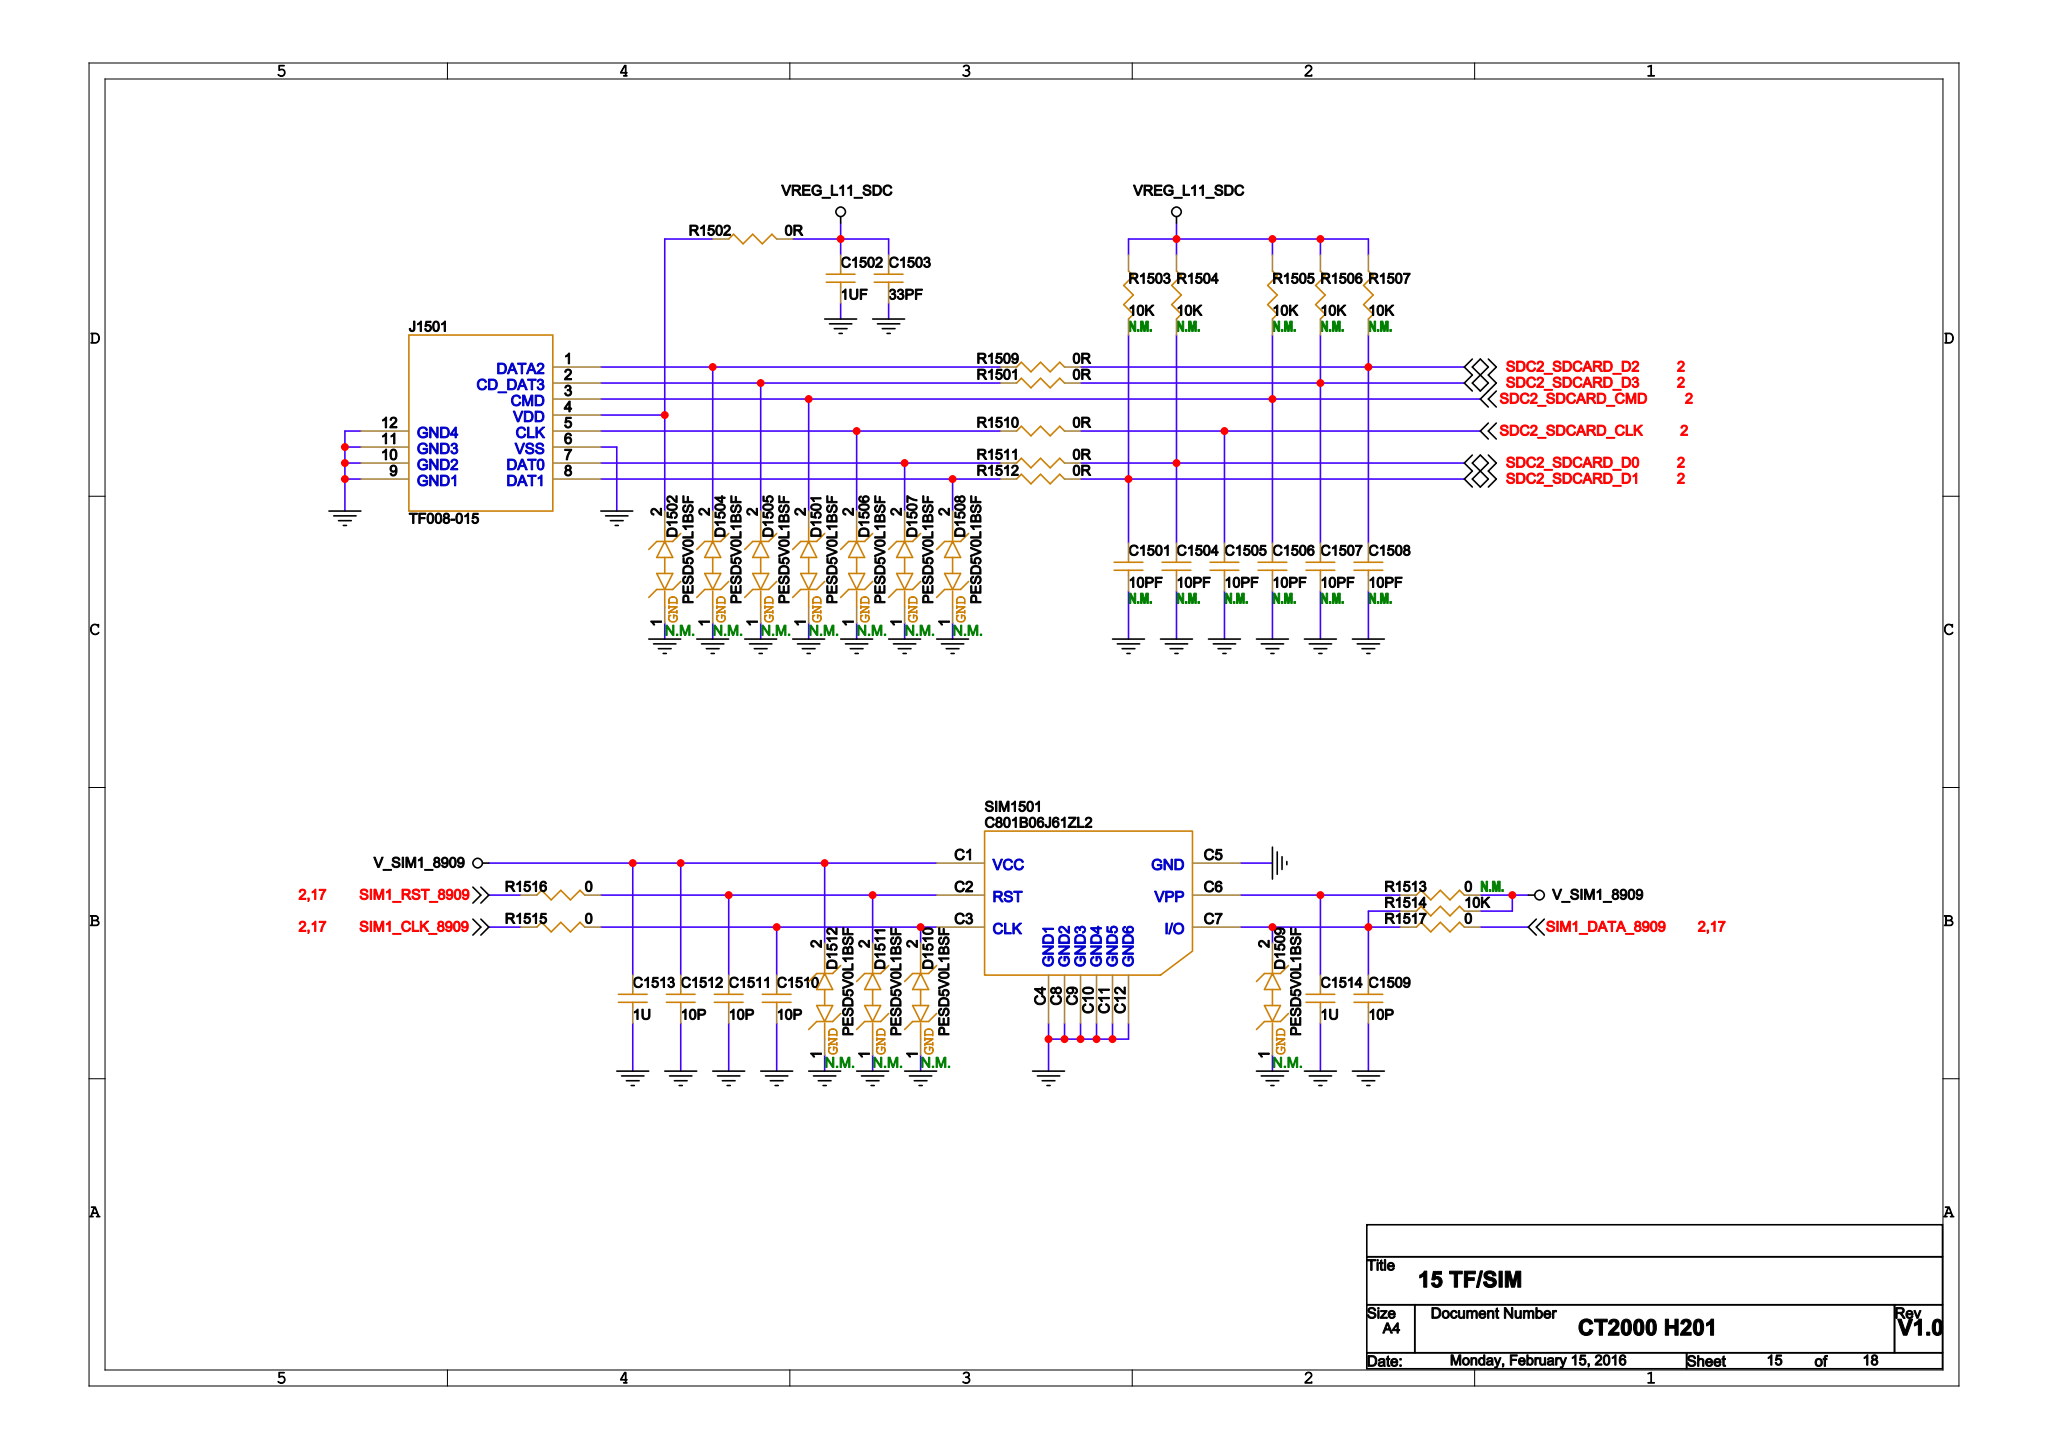Circuit board | Cadence Allegro | 573 parts | 376 nets | one sheet of the schematic
Parts on this sheet (reference | value | footprint):
C1501 | 10P | C0402
C1502 | 1U | C0402
C1503 | 33P | C0402
C1504 | 10P | C0402
C1505 | 10P | C0402
C1506 | 10P | C0402
C1507 | 10P | C0402
C1508 | 10P | C0402
C1509 | 10P | C0402
C1510 | 10P | C0402
C1511 | 10P | C0402
C1512 | 10P | C0402
C1513 | 1U | C0402
C1514 | 1U | C0402
D1501 | PESD5V0L1BSF | DSN0603-2
D1502 | PESD5V0L1BSF | DSN0603-2
D1504 | PESD5V0L1BSF | DSN0603-2
D1505 | PESD5V0L1BSF | DSN0603-2
D1506 | PESD5V0L1BSF | DSN0603-2
D1507 | PESD5V0L1BSF | DSN0603-2
D1508 | PESD5V0L1BSF | DSN0603-2
D1509 | PESD5V0L1BSF | DSN0603-2
D1510 | PESD5V0L1BSF | DSN0603-2
D1511 | PESD5V0L1BSF | DSN0603-2
D1512 | PESD5V0L1BSF | DSN0603-2
J1501 | TF008-015 | TF_TF008-015
R1501 | 0 | R0402
R1502 | 0 | R0402
R1503 | 10K | R0402
R1504 | 10K | R0402
R1505 | 10K | R0402
R1506 | 10K | R0402
R1507 | 10K | R0402
R1509 | 0 | R0402
R1510 | 0 | R0402
R1511 | 0 | R0402
R1512 | 0 | R0402
R1513 | 0 | R0402
R1514 | 10K | R0402
R1515 | 0 | R0402
R1516 | 0 | R0402
R1517 | 0 | R0402
SIM1501 | C801B06J61ZL2 | SIM_C801B06J61ZL2
Nets of these parts (net: part-pin ...):
GND: C1501-2 C1502-2 C1503-1 C1504-2 C1505-2 C1506-2 C1507-2 C1508-2 C1509-2 C1510-2 C1511-2 C1512-2 C1513-2 C1514-2 D1501-1 D1502-1 D1504-1 D1505-1 D1506-1 D1507-1 D1508-1 D1509-1 D1510-1 D1511-1 D1512-1 J1501-6 J1501-9 J1501-10 J1501-11 J1501-12 SIM1501-C4 SIM1501-C5 SIM1501-C8 SIM1501-C9 SIM1501-C10 SIM1501-C11 SIM1501-C12
N52260803: D1505-2 J1501-2 R1501-1
N52260817: D1506-2 J1501-5 R1510-1
SDC2_SDCARD_CMD: C1506-1 D1501-2 J1501-3 R1505-1
N52260821: D1507-2 J1501-7 R1511-1
N52260829: D1508-2 J1501-8 R1512-1
N52260797: D1504-2 J1501-1 R1509-1
N52260786: D1502-2 J1501-4 R1502-1
N52780212: C1510-1 D1510-2 R1515-2 SIM1501-C3
N52780081: C1509-1 D1509-2 R1514-1 R1517-1 SIM1501-C7
N52780216: C1511-1 D1511-2 R1516-2 SIM1501-C2
V_SIM1_8909: C1512-1 C1513-1 D1512-2 R1513-2 R1514-2 SIM1501-C1
N52780169: C1514-1 R1513-1 SIM1501-C6
SDC2_SDCARD_D0: C1504-1 R1504-1 R1511-2
SDC2_SDCARD_D1: C1501-1 R1503-1 R1512-2
SDC2_SDCARD_D2: C1508-1 R1507-1 R1509-2
SDC2_SDCARD_D3: C1507-1 R1501-2 R1506-1
SIM1_CLK_8909: R1515-1
SIM1_DATA_8909: R1517-2
SIM1_RST_8909: R1516-1
VREG_L11_SDC: C1502-1 C1503-2 R1502-2 R1503-2 R1504-2 R1505-2 R1506-2 R1507-2
SDC2_SDCARD_CLK: C1505-1 R1510-2